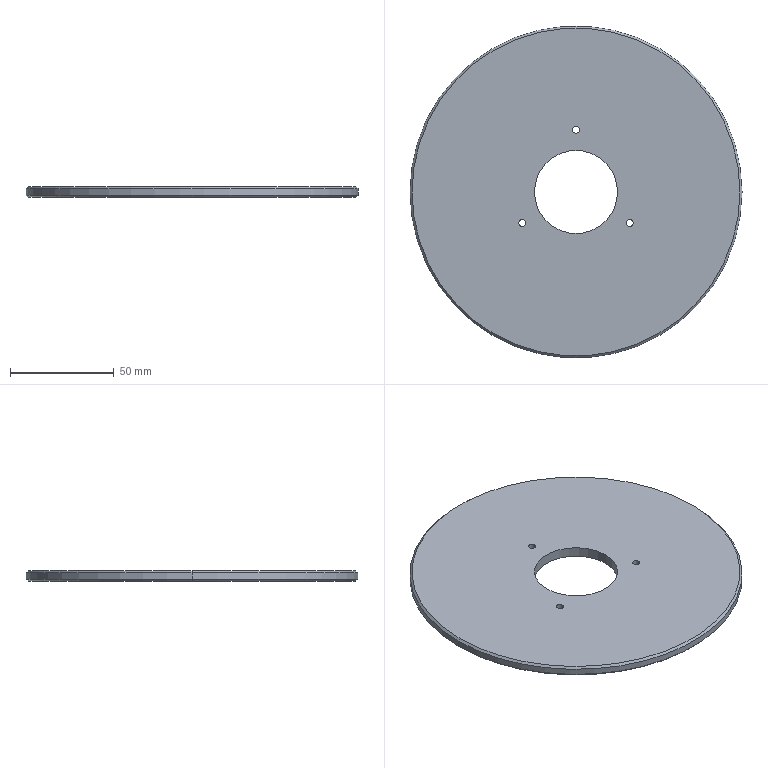Part | STEP file | 11-FG-B05311 | 1 solid | 16 faces | box 160 x 160 x 5 mm | volume 93587 mm3 | cylinder 10 | cone 4 | plane 2 | commonest cylinder face diameters 3.3 x6 40.1 x2 160 x2
STEP:
#1=CARTESIAN_POINT('',(-27.631,-15.,5.));
#2=VERTEX_POINT('',#1);
#3=CARTESIAN_POINT('',(-24.331,-15.,5.));
#4=VERTEX_POINT('',#3);
#5=CARTESIAN_POINT('',(-25.981,-15.,5.));
#6=DIRECTION('',(0.,0.,1.));
#7=DIRECTION('',(1.,0.,0.));
#8=AXIS2_PLACEMENT_3D('',#5,#6,#7);
#9=CIRCLE('',#8,1.65);
#10=EDGE_CURVE('',#2,#4,#9,.T.);
#11=ORIENTED_EDGE('',*,*,#10,.T.);
#12=CARTESIAN_POINT('',(-24.331,-15.,0.));
#13=VERTEX_POINT('',#12);
#14=CARTESIAN_POINT('',(-24.331,-15.,0.));
#15=DIRECTION('',(0.,0.,-1.));
#16=VECTOR('',#15,1000.);
#17=LINE('',#14,#16);
#18=EDGE_CURVE('',#4,#13,#17,.T.);
#19=ORIENTED_EDGE('',*,*,#18,.T.);
#20=CARTESIAN_POINT('',(-27.631,-15.,0.));
#21=VERTEX_POINT('',#20);
#22=CARTESIAN_POINT('',(-25.981,-15.,0.));
#23=DIRECTION('',(0.,0.,-1.));
#24=DIRECTION('',(-1.,0.,0.));
#25=AXIS2_PLACEMENT_3D('',#22,#23,#24);
#26=CIRCLE('',#25,1.65);
#27=EDGE_CURVE('',#13,#21,#26,.T.);
#28=ORIENTED_EDGE('',*,*,#27,.T.);
#29=CARTESIAN_POINT('',(-27.631,-15.,0.));
#30=DIRECTION('',(0.,0.,-1.));
#31=VECTOR('',#30,1000.);
#32=LINE('',#29,#31);
#33=EDGE_CURVE('',#2,#21,#32,.T.);
#34=ORIENTED_EDGE('',*,*,#33,.F.);
#35=EDGE_LOOP('',(#11,#19,#28,#34));
#36=FACE_OUTER_BOUND('',#35,.T.);
#37=CARTESIAN_POINT('',(-25.981,-15.,0.));
#38=DIRECTION('',(0.,0.,-1.));
#39=DIRECTION('',(-1.,0.,0.));
#40=AXIS2_PLACEMENT_3D('',#37,#38,#39);
#41=CYLINDRICAL_SURFACE('',#40,1.65);
#42=ADVANCED_FACE('',(#36),#41,.F.);
#43=CARTESIAN_POINT('',(24.331,-15.,5.));
#44=VERTEX_POINT('',#43);
#45=CARTESIAN_POINT('',(27.631,-15.,5.));
#46=VERTEX_POINT('',#45);
#47=CARTESIAN_POINT('',(25.981,-15.,5.));
#48=DIRECTION('',(0.,0.,1.));
#49=DIRECTION('',(1.,0.,0.));
#50=AXIS2_PLACEMENT_3D('',#47,#48,#49);
#51=CIRCLE('',#50,1.65);
#52=EDGE_CURVE('',#44,#46,#51,.T.);
#53=ORIENTED_EDGE('',*,*,#52,.T.);
#54=CARTESIAN_POINT('',(27.631,-15.,0.));
#55=VERTEX_POINT('',#54);
#56=CARTESIAN_POINT('',(27.631,-15.,0.));
#57=DIRECTION('',(0.,0.,-1.));
#58=VECTOR('',#57,1000.);
#59=LINE('',#56,#58);
#60=EDGE_CURVE('',#46,#55,#59,.T.);
#61=ORIENTED_EDGE('',*,*,#60,.T.);
#62=CARTESIAN_POINT('',(24.331,-15.,0.));
#63=VERTEX_POINT('',#62);
#64=CARTESIAN_POINT('',(25.981,-15.,0.));
#65=DIRECTION('',(0.,0.,-1.));
#66=DIRECTION('',(-1.,0.,0.));
#67=AXIS2_PLACEMENT_3D('',#64,#65,#66);
#68=CIRCLE('',#67,1.65);
#69=EDGE_CURVE('',#55,#63,#68,.T.);
#70=ORIENTED_EDGE('',*,*,#69,.T.);
#71=CARTESIAN_POINT('',(24.331,-15.,0.));
#72=DIRECTION('',(0.,0.,-1.));
#73=VECTOR('',#72,1000.);
#74=LINE('',#71,#73);
#75=EDGE_CURVE('',#44,#63,#74,.T.);
#76=ORIENTED_EDGE('',*,*,#75,.F.);
#77=EDGE_LOOP('',(#53,#61,#70,#76));
#78=FACE_OUTER_BOUND('',#77,.T.);
#79=CARTESIAN_POINT('',(25.981,-15.,0.));
#80=DIRECTION('',(0.,0.,-1.));
#81=DIRECTION('',(-1.,0.,0.));
#82=AXIS2_PLACEMENT_3D('',#79,#80,#81);
#83=CYLINDRICAL_SURFACE('',#82,1.65);
#84=ADVANCED_FACE('',(#78),#83,.F.);
#85=CARTESIAN_POINT('',(-1.65,30.,5.));
#86=VERTEX_POINT('',#85);
#87=CARTESIAN_POINT('',(1.65,30.,5.));
#88=VERTEX_POINT('',#87);
#89=CARTESIAN_POINT('',(0.,30.,5.));
#90=DIRECTION('',(0.,0.,1.));
#91=DIRECTION('',(1.,0.,0.));
#92=AXIS2_PLACEMENT_3D('',#89,#90,#91);
#93=CIRCLE('',#92,1.65);
#94=EDGE_CURVE('',#86,#88,#93,.T.);
#95=ORIENTED_EDGE('',*,*,#94,.T.);
#96=CARTESIAN_POINT('',(1.65,30.,0.));
#97=VERTEX_POINT('',#96);
#98=CARTESIAN_POINT('',(1.65,30.,0.));
#99=DIRECTION('',(0.,0.,-1.));
#100=VECTOR('',#99,1000.);
#101=LINE('',#98,#100);
#102=EDGE_CURVE('',#88,#97,#101,.T.);
#103=ORIENTED_EDGE('',*,*,#102,.T.);
#104=CARTESIAN_POINT('',(-1.65,30.,0.));
#105=VERTEX_POINT('',#104);
#106=CARTESIAN_POINT('',(0.,30.,0.));
#107=DIRECTION('',(0.,0.,-1.));
#108=DIRECTION('',(-1.,0.,0.));
#109=AXIS2_PLACEMENT_3D('',#106,#107,#108);
#110=CIRCLE('',#109,1.65);
#111=EDGE_CURVE('',#97,#105,#110,.T.);
#112=ORIENTED_EDGE('',*,*,#111,.T.);
#113=CARTESIAN_POINT('',(-1.65,30.,0.));
#114=DIRECTION('',(0.,0.,-1.));
#115=VECTOR('',#114,1000.);
#116=LINE('',#113,#115);
#117=EDGE_CURVE('',#86,#105,#116,.T.);
#118=ORIENTED_EDGE('',*,*,#117,.F.);
#119=EDGE_LOOP('',(#95,#103,#112,#118));
#120=FACE_OUTER_BOUND('',#119,.T.);
#121=CARTESIAN_POINT('',(0.,30.,0.));
#122=DIRECTION('',(0.,0.,-1.));
#123=DIRECTION('',(-1.,0.,0.));
#124=AXIS2_PLACEMENT_3D('',#121,#122,#123);
#125=CYLINDRICAL_SURFACE('',#124,1.65);
#126=ADVANCED_FACE('',(#120),#125,.F.);
#127=CARTESIAN_POINT('',(20.05,0.,5.));
#128=VERTEX_POINT('',#127);
#129=CARTESIAN_POINT('',(-20.05,0.,5.));
#130=VERTEX_POINT('',#129);
#131=CARTESIAN_POINT('',(0.,0.,5.));
#132=DIRECTION('',(0.,0.,-1.));
#133=DIRECTION('',(-1.,0.,0.));
#134=AXIS2_PLACEMENT_3D('',#131,#132,#133);
#135=CIRCLE('',#134,20.05);
#136=EDGE_CURVE('',#128,#130,#135,.T.);
#137=ORIENTED_EDGE('',*,*,#136,.F.);
#138=CARTESIAN_POINT('',(20.05,0.,0.));
#139=VERTEX_POINT('',#138);
#140=CARTESIAN_POINT('',(20.05,0.,5.));
#141=DIRECTION('',(0.,0.,-1.));
#142=VECTOR('',#141,1000.);
#143=LINE('',#140,#142);
#144=EDGE_CURVE('',#128,#139,#143,.T.);
#145=ORIENTED_EDGE('',*,*,#144,.T.);
#146=CARTESIAN_POINT('',(-20.05,0.,0.));
#147=VERTEX_POINT('',#146);
#148=CARTESIAN_POINT('',(0.,0.,0.));
#149=DIRECTION('',(0.,0.,-1.));
#150=DIRECTION('',(-1.,0.,0.));
#151=AXIS2_PLACEMENT_3D('',#148,#149,#150);
#152=CIRCLE('',#151,20.05);
#153=EDGE_CURVE('',#139,#147,#152,.T.);
#154=ORIENTED_EDGE('',*,*,#153,.T.);
#155=CARTESIAN_POINT('',(-20.05,0.,5.));
#156=DIRECTION('',(0.,0.,-1.));
#157=VECTOR('',#156,1000.);
#158=LINE('',#155,#157);
#159=EDGE_CURVE('',#130,#147,#158,.T.);
#160=ORIENTED_EDGE('',*,*,#159,.F.);
#161=EDGE_LOOP('',(#137,#145,#154,#160));
#162=FACE_OUTER_BOUND('',#161,.T.);
#163=CARTESIAN_POINT('',(0.,0.,5.));
#164=DIRECTION('',(0.,0.,-1.));
#165=DIRECTION('',(-1.,0.,0.));
#166=AXIS2_PLACEMENT_3D('',#163,#164,#165);
#167=CYLINDRICAL_SURFACE('',#166,20.05);
#168=ADVANCED_FACE('',(#162),#167,.F.);
#169=CARTESIAN_POINT('',(79.,0.,5.));
#170=VERTEX_POINT('',#169);
#171=CARTESIAN_POINT('',(-79.,0.,5.));
#172=VERTEX_POINT('',#171);
#173=CARTESIAN_POINT('',(0.,0.,5.));
#174=DIRECTION('',(0.,0.,1.));
#175=DIRECTION('',(1.,0.,0.));
#176=AXIS2_PLACEMENT_3D('',#173,#174,#175);
#177=CIRCLE('',#176,79.);
#178=EDGE_CURVE('',#170,#172,#177,.T.);
#179=ORIENTED_EDGE('',*,*,#178,.F.);
#180=CARTESIAN_POINT('',(80.,0.,4.));
#181=VERTEX_POINT('',#180);
#182=CARTESIAN_POINT('',(79.,0.,5.));
#183=DIRECTION('',(0.7071,0.,-0.7071));
#184=VECTOR('',#183,1000.);
#185=LINE('',#182,#184);
#186=EDGE_CURVE('',#170,#181,#185,.T.);
#187=ORIENTED_EDGE('',*,*,#186,.T.);
#188=CARTESIAN_POINT('',(-80.,0.,4.));
#189=VERTEX_POINT('',#188);
#190=CARTESIAN_POINT('',(0.,0.,4.));
#191=DIRECTION('',(0.,0.,-1.));
#192=DIRECTION('',(1.,0.,0.));
#193=AXIS2_PLACEMENT_3D('',#190,#191,#192);
#194=CIRCLE('',#193,80.);
#195=EDGE_CURVE('',#189,#181,#194,.T.);
#196=ORIENTED_EDGE('',*,*,#195,.F.);
#197=CARTESIAN_POINT('',(-79.,0.,5.));
#198=DIRECTION('',(-0.7071,0.,-0.7071));
#199=VECTOR('',#198,1000.);
#200=LINE('',#197,#199);
#201=EDGE_CURVE('',#172,#189,#200,.T.);
#202=ORIENTED_EDGE('',*,*,#201,.F.);
#203=EDGE_LOOP('',(#179,#187,#196,#202));
#204=FACE_OUTER_BOUND('',#203,.T.);
#205=CARTESIAN_POINT('',(0.,0.,5.));
#206=DIRECTION('',(0.,0.,-1.));
#207=DIRECTION('',(-1.,0.,0.));
#208=AXIS2_PLACEMENT_3D('',#205,#206,#207);
#209=CONICAL_SURFACE('',#208,79.,0.7854);
#210=ADVANCED_FACE('',(#204),#209,.T.);
#211=CARTESIAN_POINT('',(-79.,0.,0.));
#212=VERTEX_POINT('',#211);
#213=CARTESIAN_POINT('',(79.,0.,0.));
#214=VERTEX_POINT('',#213);
#215=CARTESIAN_POINT('',(0.,0.,0.));
#216=DIRECTION('',(0.,0.,-1.));
#217=DIRECTION('',(1.,0.,0.));
#218=AXIS2_PLACEMENT_3D('',#215,#216,#217);
#219=CIRCLE('',#218,79.);
#220=EDGE_CURVE('',#212,#214,#219,.T.);
#221=ORIENTED_EDGE('',*,*,#220,.F.);
#222=CARTESIAN_POINT('',(-80.,0.,1.));
#223=VERTEX_POINT('',#222);
#224=CARTESIAN_POINT('',(-80.,0.,1.));
#225=DIRECTION('',(-0.7071,0.,0.7071));
#226=VECTOR('',#225,1000.);
#227=LINE('',#224,#226);
#228=EDGE_CURVE('',#212,#223,#227,.T.);
#229=ORIENTED_EDGE('',*,*,#228,.T.);
#230=CARTESIAN_POINT('',(80.,0.,1.));
#231=VERTEX_POINT('',#230);
#232=CARTESIAN_POINT('',(0.,0.,1.));
#233=DIRECTION('',(0.,0.,1.));
#234=DIRECTION('',(1.,0.,0.));
#235=AXIS2_PLACEMENT_3D('',#232,#233,#234);
#236=CIRCLE('',#235,80.);
#237=EDGE_CURVE('',#231,#223,#236,.T.);
#238=ORIENTED_EDGE('',*,*,#237,.F.);
#239=CARTESIAN_POINT('',(80.,0.,1.));
#240=DIRECTION('',(0.7071,0.,0.7071));
#241=VECTOR('',#240,1000.);
#242=LINE('',#239,#241);
#243=EDGE_CURVE('',#214,#231,#242,.T.);
#244=ORIENTED_EDGE('',*,*,#243,.F.);
#245=EDGE_LOOP('',(#221,#229,#238,#244));
#246=FACE_OUTER_BOUND('',#245,.T.);
#247=CARTESIAN_POINT('',(0.,0.,1.));
#248=DIRECTION('',(0.,0.,1.));
#249=DIRECTION('',(1.,0.,0.));
#250=AXIS2_PLACEMENT_3D('',#247,#248,#249);
#251=CONICAL_SURFACE('',#250,80.,0.7854);
#252=ADVANCED_FACE('',(#246),#251,.T.);
#253=ORIENTED_EDGE('',*,*,#195,.T.);
#254=CARTESIAN_POINT('',(80.,0.,5.));
#255=DIRECTION('',(0.,0.,-1.));
#256=VECTOR('',#255,1000.);
#257=LINE('',#254,#256);
#258=EDGE_CURVE('',#181,#231,#257,.T.);
#259=ORIENTED_EDGE('',*,*,#258,.T.);
#260=ORIENTED_EDGE('',*,*,#237,.T.);
#261=CARTESIAN_POINT('',(-80.,0.,5.));
#262=DIRECTION('',(0.,0.,-1.));
#263=VECTOR('',#262,1000.);
#264=LINE('',#261,#263);
#265=EDGE_CURVE('',#189,#223,#264,.T.);
#266=ORIENTED_EDGE('',*,*,#265,.F.);
#267=EDGE_LOOP('',(#253,#259,#260,#266));
#268=FACE_OUTER_BOUND('',#267,.T.);
#269=CARTESIAN_POINT('',(0.,0.,5.));
#270=DIRECTION('',(0.,0.,-1.));
#271=DIRECTION('',(-1.,0.,0.));
#272=AXIS2_PLACEMENT_3D('',#269,#270,#271);
#273=CYLINDRICAL_SURFACE('',#272,80.);
#274=ADVANCED_FACE('',(#268),#273,.T.);
#275=ORIENTED_EDGE('',*,*,#258,.F.);
#276=CARTESIAN_POINT('',(0.,0.,4.));
#277=DIRECTION('',(0.,0.,-1.));
#278=DIRECTION('',(1.,0.,0.));
#279=AXIS2_PLACEMENT_3D('',#276,#277,#278);
#280=CIRCLE('',#279,80.);
#281=EDGE_CURVE('',#181,#189,#280,.T.);
#282=ORIENTED_EDGE('',*,*,#281,.T.);
#283=ORIENTED_EDGE('',*,*,#265,.T.);
#284=CARTESIAN_POINT('',(0.,0.,1.));
#285=DIRECTION('',(0.,0.,1.));
#286=DIRECTION('',(1.,0.,0.));
#287=AXIS2_PLACEMENT_3D('',#284,#285,#286);
#288=CIRCLE('',#287,80.);
#289=EDGE_CURVE('',#223,#231,#288,.T.);
#290=ORIENTED_EDGE('',*,*,#289,.T.);
#291=EDGE_LOOP('',(#275,#282,#283,#290));
#292=FACE_OUTER_BOUND('',#291,.T.);
#293=CARTESIAN_POINT('',(0.,0.,5.));
#294=DIRECTION('',(0.,0.,-1.));
#295=DIRECTION('',(-1.,0.,0.));
#296=AXIS2_PLACEMENT_3D('',#293,#294,#295);
#297=CYLINDRICAL_SURFACE('',#296,80.);
#298=ADVANCED_FACE('',(#292),#297,.T.);
#299=ORIENTED_EDGE('',*,*,#10,.F.);
#300=CARTESIAN_POINT('',(-25.981,-15.,5.));
#301=DIRECTION('',(0.,0.,1.));
#302=DIRECTION('',(1.,0.,0.));
#303=AXIS2_PLACEMENT_3D('',#300,#301,#302);
#304=CIRCLE('',#303,1.65);
#305=EDGE_CURVE('',#4,#2,#304,.T.);
#306=ORIENTED_EDGE('',*,*,#305,.F.);
#307=EDGE_LOOP('',(#299,#306));
#308=FACE_BOUND('',#307,.T.);
#309=ORIENTED_EDGE('',*,*,#52,.F.);
#310=CARTESIAN_POINT('',(25.981,-15.,5.));
#311=DIRECTION('',(0.,0.,1.));
#312=DIRECTION('',(1.,0.,0.));
#313=AXIS2_PLACEMENT_3D('',#310,#311,#312);
#314=CIRCLE('',#313,1.65);
#315=EDGE_CURVE('',#46,#44,#314,.T.);
#316=ORIENTED_EDGE('',*,*,#315,.F.);
#317=EDGE_LOOP('',(#309,#316));
#318=FACE_BOUND('',#317,.T.);
#319=ORIENTED_EDGE('',*,*,#94,.F.);
#320=CARTESIAN_POINT('',(0.,30.,5.));
#321=DIRECTION('',(0.,0.,1.));
#322=DIRECTION('',(1.,0.,0.));
#323=AXIS2_PLACEMENT_3D('',#320,#321,#322);
#324=CIRCLE('',#323,1.65);
#325=EDGE_CURVE('',#88,#86,#324,.T.);
#326=ORIENTED_EDGE('',*,*,#325,.F.);
#327=EDGE_LOOP('',(#319,#326));
#328=FACE_BOUND('',#327,.T.);
#329=CARTESIAN_POINT('',(0.,0.,5.));
#330=DIRECTION('',(0.,0.,-1.));
#331=DIRECTION('',(-1.,0.,0.));
#332=AXIS2_PLACEMENT_3D('',#329,#330,#331);
#333=CIRCLE('',#332,20.05);
#334=EDGE_CURVE('',#130,#128,#333,.T.);
#335=ORIENTED_EDGE('',*,*,#334,.T.);
#336=ORIENTED_EDGE('',*,*,#136,.T.);
#337=EDGE_LOOP('',(#335,#336));
#338=FACE_BOUND('',#337,.T.);
#339=CARTESIAN_POINT('',(0.,0.,5.));
#340=DIRECTION('',(0.,0.,1.));
#341=DIRECTION('',(1.,0.,0.));
#342=AXIS2_PLACEMENT_3D('',#339,#340,#341);
#343=CIRCLE('',#342,79.);
#344=EDGE_CURVE('',#172,#170,#343,.T.);
#345=ORIENTED_EDGE('',*,*,#344,.T.);
#346=ORIENTED_EDGE('',*,*,#178,.T.);
#347=EDGE_LOOP('',(#345,#346));
#348=FACE_OUTER_BOUND('',#347,.T.);
#349=CARTESIAN_POINT('',(0.,0.,5.));
#350=DIRECTION('',(0.,0.,1.));
#351=DIRECTION('',(1.,0.,0.));
#352=AXIS2_PLACEMENT_3D('',#349,#350,#351);
#353=PLANE('',#352);
#354=ADVANCED_FACE('',(#308,#318,#328,#338,#348),#353,.T.);
#355=CARTESIAN_POINT('',(-25.981,-15.,0.));
#356=DIRECTION('',(0.,0.,-1.));
#357=DIRECTION('',(-1.,0.,0.));
#358=AXIS2_PLACEMENT_3D('',#355,#356,#357);
#359=CIRCLE('',#358,1.65);
#360=EDGE_CURVE('',#21,#13,#359,.T.);
#361=ORIENTED_EDGE('',*,*,#360,.F.);
#362=ORIENTED_EDGE('',*,*,#27,.F.);
#363=EDGE_LOOP('',(#361,#362));
#364=FACE_BOUND('',#363,.T.);
#365=CARTESIAN_POINT('',(25.981,-15.,0.));
#366=DIRECTION('',(0.,0.,-1.));
#367=DIRECTION('',(-1.,0.,0.));
#368=AXIS2_PLACEMENT_3D('',#365,#366,#367);
#369=CIRCLE('',#368,1.65);
#370=EDGE_CURVE('',#63,#55,#369,.T.);
#371=ORIENTED_EDGE('',*,*,#370,.F.);
#372=ORIENTED_EDGE('',*,*,#69,.F.);
#373=EDGE_LOOP('',(#371,#372));
#374=FACE_BOUND('',#373,.T.);
#375=CARTESIAN_POINT('',(0.,30.,0.));
#376=DIRECTION('',(0.,0.,-1.));
#377=DIRECTION('',(-1.,0.,0.));
#378=AXIS2_PLACEMENT_3D('',#375,#376,#377);
#379=CIRCLE('',#378,1.65);
#380=EDGE_CURVE('',#105,#97,#379,.T.);
#381=ORIENTED_EDGE('',*,*,#380,.F.);
#382=ORIENTED_EDGE('',*,*,#111,.F.);
#383=EDGE_LOOP('',(#381,#382));
#384=FACE_BOUND('',#383,.T.);
#385=CARTESIAN_POINT('',(0.,0.,0.));
#386=DIRECTION('',(0.,0.,-1.));
#387=DIRECTION('',(-1.,0.,0.));
#388=AXIS2_PLACEMENT_3D('',#385,#386,#387);
#389=CIRCLE('',#388,20.05);
#390=EDGE_CURVE('',#147,#139,#389,.T.);
#391=ORIENTED_EDGE('',*,*,#390,.F.);
#392=ORIENTED_EDGE('',*,*,#153,.F.);
#393=EDGE_LOOP('',(#391,#392));
#394=FACE_BOUND('',#393,.T.);
#395=CARTESIAN_POINT('',(0.,0.,0.));
#396=DIRECTION('',(0.,0.,-1.));
#397=DIRECTION('',(1.,0.,0.));
#398=AXIS2_PLACEMENT_3D('',#395,#396,#397);
#399=CIRCLE('',#398,79.);
#400=EDGE_CURVE('',#214,#212,#399,.T.);
#401=ORIENTED_EDGE('',*,*,#400,.T.);
#402=ORIENTED_EDGE('',*,*,#220,.T.);
#403=EDGE_LOOP('',(#401,#402));
#404=FACE_OUTER_BOUND('',#403,.T.);
#405=CARTESIAN_POINT('',(0.,0.,0.));
#406=DIRECTION('',(0.,0.,1.));
#407=DIRECTION('',(1.,0.,0.));
#408=AXIS2_PLACEMENT_3D('',#405,#406,#407);
#409=PLANE('',#408);
#410=ADVANCED_FACE('',(#364,#374,#384,#394,#404),#409,.F.);
#411=ORIENTED_EDGE('',*,*,#228,.F.);
#412=ORIENTED_EDGE('',*,*,#400,.F.);
#413=ORIENTED_EDGE('',*,*,#243,.T.);
#414=ORIENTED_EDGE('',*,*,#289,.F.);
#415=EDGE_LOOP('',(#411,#412,#413,#414));
#416=FACE_OUTER_BOUND('',#415,.T.);
#417=CARTESIAN_POINT('',(0.,0.,1.));
#418=DIRECTION('',(0.,0.,1.));
#419=DIRECTION('',(1.,0.,0.));
#420=AXIS2_PLACEMENT_3D('',#417,#418,#419);
#421=CONICAL_SURFACE('',#420,80.,0.7854);
#422=ADVANCED_FACE('',(#416),#421,.T.);
#423=ORIENTED_EDGE('',*,*,#186,.F.);
#424=ORIENTED_EDGE('',*,*,#344,.F.);
#425=ORIENTED_EDGE('',*,*,#201,.T.);
#426=ORIENTED_EDGE('',*,*,#281,.F.);
#427=EDGE_LOOP('',(#423,#424,#425,#426));
#428=FACE_OUTER_BOUND('',#427,.T.);
#429=CARTESIAN_POINT('',(0.,0.,5.));
#430=DIRECTION('',(0.,0.,-1.));
#431=DIRECTION('',(-1.,0.,0.));
#432=AXIS2_PLACEMENT_3D('',#429,#430,#431);
#433=CONICAL_SURFACE('',#432,79.,0.7854);
#434=ADVANCED_FACE('',(#428),#433,.T.);
#435=ORIENTED_EDGE('',*,*,#144,.F.);
#436=ORIENTED_EDGE('',*,*,#334,.F.);
#437=ORIENTED_EDGE('',*,*,#159,.T.);
#438=ORIENTED_EDGE('',*,*,#390,.T.);
#439=EDGE_LOOP('',(#435,#436,#437,#438));
#440=FACE_OUTER_BOUND('',#439,.T.);
#441=CARTESIAN_POINT('',(0.,0.,5.));
#442=DIRECTION('',(0.,0.,-1.));
#443=DIRECTION('',(-1.,0.,0.));
#444=AXIS2_PLACEMENT_3D('',#441,#442,#443);
#445=CYLINDRICAL_SURFACE('',#444,20.05);
#446=ADVANCED_FACE('',(#440),#445,.F.);
#447=ORIENTED_EDGE('',*,*,#102,.F.);
#448=ORIENTED_EDGE('',*,*,#325,.T.);
#449=ORIENTED_EDGE('',*,*,#117,.T.);
#450=ORIENTED_EDGE('',*,*,#380,.T.);
#451=EDGE_LOOP('',(#447,#448,#449,#450));
#452=FACE_OUTER_BOUND('',#451,.T.);
#453=CARTESIAN_POINT('',(0.,30.,0.));
#454=DIRECTION('',(0.,0.,-1.));
#455=DIRECTION('',(-1.,0.,0.));
#456=AXIS2_PLACEMENT_3D('',#453,#454,#455);
#457=CYLINDRICAL_SURFACE('',#456,1.65);
#458=ADVANCED_FACE('',(#452),#457,.F.);
#459=ORIENTED_EDGE('',*,*,#60,.F.);
#460=ORIENTED_EDGE('',*,*,#315,.T.);
#461=ORIENTED_EDGE('',*,*,#75,.T.);
#462=ORIENTED_EDGE('',*,*,#370,.T.);
#463=EDGE_LOOP('',(#459,#460,#461,#462));
#464=FACE_OUTER_BOUND('',#463,.T.);
#465=CARTESIAN_POINT('',(25.981,-15.,0.));
#466=DIRECTION('',(0.,0.,-1.));
#467=DIRECTION('',(-1.,0.,0.));
#468=AXIS2_PLACEMENT_3D('',#465,#466,#467);
#469=CYLINDRICAL_SURFACE('',#468,1.65);
#470=ADVANCED_FACE('',(#464),#469,.F.);
#471=ORIENTED_EDGE('',*,*,#18,.F.);
#472=ORIENTED_EDGE('',*,*,#305,.T.);
#473=ORIENTED_EDGE('',*,*,#33,.T.);
#474=ORIENTED_EDGE('',*,*,#360,.T.);
#475=EDGE_LOOP('',(#471,#472,#473,#474));
#476=FACE_OUTER_BOUND('',#475,.T.);
#477=CARTESIAN_POINT('',(-25.981,-15.,0.));
#478=DIRECTION('',(0.,0.,-1.));
#479=DIRECTION('',(-1.,0.,0.));
#480=AXIS2_PLACEMENT_3D('',#477,#478,#479);
#481=CYLINDRICAL_SURFACE('',#480,1.65);
#482=ADVANCED_FACE('',(#476),#481,.F.);
#483=CLOSED_SHELL('',(#42,#84,#126,#168,#210,#252,#274,#298,#354,#410,#422,#434,#446,#458,#470,#482));
#484=MANIFOLD_SOLID_BREP('',#483);
#485=CARTESIAN_POINT('',(0.,0.,0.));
#486=DIRECTION('',(0.,0.,1.));
#487=DIRECTION('',(1.,0.,0.));
#488=AXIS2_PLACEMENT_3D('',#485,#486,#487);
#489=(LENGTH_UNIT()NAMED_UNIT(*)SI_UNIT(.MILLI.,.METRE.));
#490=UNCERTAINTY_MEASURE_WITH_UNIT(LENGTH_MEASURE(0.00001),#489,'','');
#491=(NAMED_UNIT(*)PLANE_ANGLE_UNIT()SI_UNIT($,.RADIAN.));
#492=(NAMED_UNIT(*)SI_UNIT($,.STERADIAN.)SOLID_ANGLE_UNIT());
#493=(GEOMETRIC_REPRESENTATION_CONTEXT(3)GLOBAL_UNCERTAINTY_ASSIGNED_CONTEXT((#490))GLOBAL_UNIT_ASSIGNED_CONTEXT((#489,#491,#492))REPRESENTATION_CONTEXT('',''));
#494=ADVANCED_BREP_SHAPE_REPRESENTATION('',(#484,#488),#493);